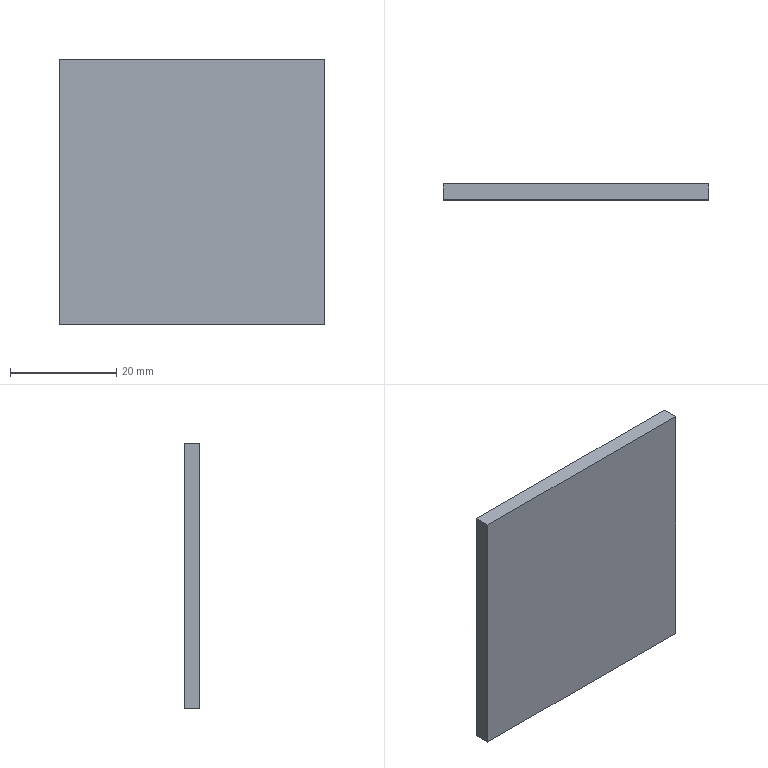Part | SolidWorks | features Extrusion 1 | 1 solid | 6 faces | box 50 x 3 x 50 mm | volume 7500 mm3 | plane 6
STEP:
#1=CARTESIAN_POINT('',(25.,0.,25.));
#2=VERTEX_POINT('',#1);
#3=CARTESIAN_POINT('',(25.,0.,-25.));
#4=VERTEX_POINT('',#3);
#5=CARTESIAN_POINT('',(25.,0.,25.));
#6=DIRECTION('',(0.,0.,-1.));
#7=VECTOR('',#6,1000.);
#8=LINE('',#5,#7);
#9=EDGE_CURVE('',#2,#4,#8,.T.);
#10=ORIENTED_EDGE('',*,*,#9,.T.);
#11=CARTESIAN_POINT('',(25.,3.,-25.));
#12=VERTEX_POINT('',#11);
#13=CARTESIAN_POINT('',(25.,3.,-25.));
#14=DIRECTION('',(0.,-1.,0.));
#15=VECTOR('',#14,1000.);
#16=LINE('',#13,#15);
#17=EDGE_CURVE('',#12,#4,#16,.T.);
#18=ORIENTED_EDGE('',*,*,#17,.F.);
#19=CARTESIAN_POINT('',(25.,3.,25.));
#20=VERTEX_POINT('',#19);
#21=CARTESIAN_POINT('',(25.,3.,25.));
#22=DIRECTION('',(0.,0.,-1.));
#23=VECTOR('',#22,1000.);
#24=LINE('',#21,#23);
#25=EDGE_CURVE('',#20,#12,#24,.T.);
#26=ORIENTED_EDGE('',*,*,#25,.F.);
#27=CARTESIAN_POINT('',(25.,3.,25.));
#28=DIRECTION('',(0.,-1.,0.));
#29=VECTOR('',#28,1000.);
#30=LINE('',#27,#29);
#31=EDGE_CURVE('',#20,#2,#30,.T.);
#32=ORIENTED_EDGE('',*,*,#31,.T.);
#33=EDGE_LOOP('',(#10,#18,#26,#32));
#34=FACE_OUTER_BOUND('',#33,.T.);
#35=CARTESIAN_POINT('',(25.,3.,25.));
#36=DIRECTION('',(-1.,0.,0.));
#37=DIRECTION('',(0.,0.,1.));
#38=AXIS2_PLACEMENT_3D('',#35,#36,#37);
#39=PLANE('',#38);
#40=ADVANCED_FACE('',(#34),#39,.F.);
#41=CARTESIAN_POINT('',(-25.,0.,-25.));
#42=VERTEX_POINT('',#41);
#43=CARTESIAN_POINT('',(-25.,0.,-25.));
#44=DIRECTION('',(-1.,0.,0.));
#45=VECTOR('',#44,1000.);
#46=LINE('',#43,#45);
#47=EDGE_CURVE('',#4,#42,#46,.T.);
#48=ORIENTED_EDGE('',*,*,#47,.T.);
#49=CARTESIAN_POINT('',(-25.,3.,-25.));
#50=VERTEX_POINT('',#49);
#51=CARTESIAN_POINT('',(-25.,3.,-25.));
#52=DIRECTION('',(0.,-1.,0.));
#53=VECTOR('',#52,1000.);
#54=LINE('',#51,#53);
#55=EDGE_CURVE('',#50,#42,#54,.T.);
#56=ORIENTED_EDGE('',*,*,#55,.F.);
#57=CARTESIAN_POINT('',(-25.,3.,-25.));
#58=DIRECTION('',(-1.,0.,0.));
#59=VECTOR('',#58,1000.);
#60=LINE('',#57,#59);
#61=EDGE_CURVE('',#12,#50,#60,.T.);
#62=ORIENTED_EDGE('',*,*,#61,.F.);
#63=ORIENTED_EDGE('',*,*,#17,.T.);
#64=EDGE_LOOP('',(#48,#56,#62,#63));
#65=FACE_OUTER_BOUND('',#64,.T.);
#66=CARTESIAN_POINT('',(-25.,3.,-25.));
#67=DIRECTION('',(0.,0.,1.));
#68=DIRECTION('',(1.,0.,0.));
#69=AXIS2_PLACEMENT_3D('',#66,#67,#68);
#70=PLANE('',#69);
#71=ADVANCED_FACE('',(#65),#70,.F.);
#72=CARTESIAN_POINT('',(-25.,0.,25.));
#73=VERTEX_POINT('',#72);
#74=CARTESIAN_POINT('',(-25.,0.,25.));
#75=DIRECTION('',(0.,0.,1.));
#76=VECTOR('',#75,1000.);
#77=LINE('',#74,#76);
#78=EDGE_CURVE('',#42,#73,#77,.T.);
#79=ORIENTED_EDGE('',*,*,#78,.T.);
#80=CARTESIAN_POINT('',(-25.,3.,25.));
#81=VERTEX_POINT('',#80);
#82=CARTESIAN_POINT('',(-25.,3.,25.));
#83=DIRECTION('',(0.,-1.,0.));
#84=VECTOR('',#83,1000.);
#85=LINE('',#82,#84);
#86=EDGE_CURVE('',#81,#73,#85,.T.);
#87=ORIENTED_EDGE('',*,*,#86,.F.);
#88=CARTESIAN_POINT('',(-25.,3.,25.));
#89=DIRECTION('',(0.,0.,1.));
#90=VECTOR('',#89,1000.);
#91=LINE('',#88,#90);
#92=EDGE_CURVE('',#50,#81,#91,.T.);
#93=ORIENTED_EDGE('',*,*,#92,.F.);
#94=ORIENTED_EDGE('',*,*,#55,.T.);
#95=EDGE_LOOP('',(#79,#87,#93,#94));
#96=FACE_OUTER_BOUND('',#95,.T.);
#97=CARTESIAN_POINT('',(-25.,3.,25.));
#98=DIRECTION('',(1.,0.,0.));
#99=DIRECTION('',(0.,0.,-1.));
#100=AXIS2_PLACEMENT_3D('',#97,#98,#99);
#101=PLANE('',#100);
#102=ADVANCED_FACE('',(#96),#101,.F.);
#103=CARTESIAN_POINT('',(-25.,0.,25.));
#104=DIRECTION('',(1.,0.,0.));
#105=VECTOR('',#104,1000.);
#106=LINE('',#103,#105);
#107=EDGE_CURVE('',#73,#2,#106,.T.);
#108=ORIENTED_EDGE('',*,*,#107,.T.);
#109=ORIENTED_EDGE('',*,*,#31,.F.);
#110=CARTESIAN_POINT('',(-25.,3.,25.));
#111=DIRECTION('',(1.,0.,0.));
#112=VECTOR('',#111,1000.);
#113=LINE('',#110,#112);
#114=EDGE_CURVE('',#81,#20,#113,.T.);
#115=ORIENTED_EDGE('',*,*,#114,.F.);
#116=ORIENTED_EDGE('',*,*,#86,.T.);
#117=EDGE_LOOP('',(#108,#109,#115,#116));
#118=FACE_OUTER_BOUND('',#117,.T.);
#119=CARTESIAN_POINT('',(-25.,3.,25.));
#120=DIRECTION('',(0.,0.,-1.));
#121=DIRECTION('',(-1.,0.,0.));
#122=AXIS2_PLACEMENT_3D('',#119,#120,#121);
#123=PLANE('',#122);
#124=ADVANCED_FACE('',(#118),#123,.F.);
#125=ORIENTED_EDGE('',*,*,#25,.T.);
#126=ORIENTED_EDGE('',*,*,#61,.T.);
#127=ORIENTED_EDGE('',*,*,#92,.T.);
#128=ORIENTED_EDGE('',*,*,#114,.T.);
#129=EDGE_LOOP('',(#125,#126,#127,#128));
#130=FACE_OUTER_BOUND('',#129,.T.);
#131=CARTESIAN_POINT('',(0.,3.,0.));
#132=DIRECTION('',(0.,-1.,0.));
#133=DIRECTION('',(0.,0.,-1.));
#134=AXIS2_PLACEMENT_3D('',#131,#132,#133);
#135=PLANE('',#134);
#136=ADVANCED_FACE('',(#130),#135,.F.);
#137=ORIENTED_EDGE('',*,*,#9,.F.);
#138=ORIENTED_EDGE('',*,*,#107,.F.);
#139=ORIENTED_EDGE('',*,*,#78,.F.);
#140=ORIENTED_EDGE('',*,*,#47,.F.);
#141=EDGE_LOOP('',(#137,#138,#139,#140));
#142=FACE_OUTER_BOUND('',#141,.T.);
#143=CARTESIAN_POINT('',(0.,0.,0.));
#144=DIRECTION('',(0.,-1.,0.));
#145=DIRECTION('',(0.,0.,-1.));
#146=AXIS2_PLACEMENT_3D('',#143,#144,#145);
#147=PLANE('',#146);
#148=ADVANCED_FACE('',(#142),#147,.T.);
#149=CLOSED_SHELL('',(#40,#71,#102,#124,#136,#148));
#150=MANIFOLD_SOLID_BREP('',#149);
#151=CARTESIAN_POINT('',(0.,0.,0.));
#152=DIRECTION('',(0.,0.,1.));
#153=DIRECTION('',(1.,0.,0.));
#154=AXIS2_PLACEMENT_3D('',#151,#152,#153);
#155=(LENGTH_UNIT()NAMED_UNIT(*)SI_UNIT(.MILLI.,.METRE.));
#156=UNCERTAINTY_MEASURE_WITH_UNIT(LENGTH_MEASURE(0.00001),#155,'','');
#157=(NAMED_UNIT(*)PLANE_ANGLE_UNIT()SI_UNIT($,.RADIAN.));
#158=(NAMED_UNIT(*)SI_UNIT($,.STERADIAN.)SOLID_ANGLE_UNIT());
#159=(GEOMETRIC_REPRESENTATION_CONTEXT(3)GLOBAL_UNCERTAINTY_ASSIGNED_CONTEXT((#156))GLOBAL_UNIT_ASSIGNED_CONTEXT((#155,#157,#158))REPRESENTATION_CONTEXT('',''));
#160=ADVANCED_BREP_SHAPE_REPRESENTATION('',(#150,#154),#159);